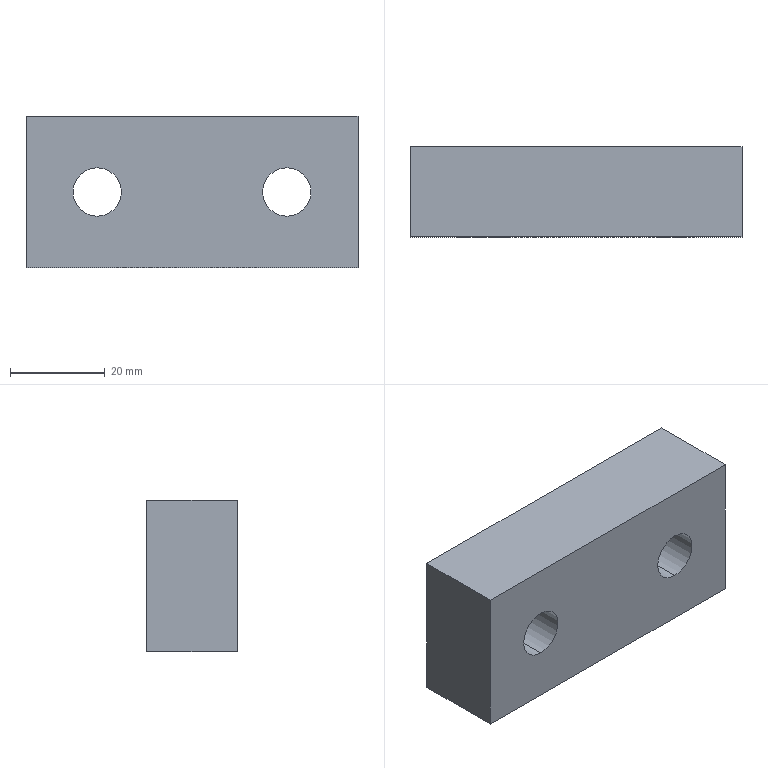Part | SolidWorks | features FlatPattern 1, HoleWzd 1, SMBaseFlange 1, SheetMetal 1 | 1 solid | 10 faces | box 70 x 19 x 32 mm | volume 39455 mm3 | plane 6 | cylinder 4 | commonest cylinder face diameters 10.2 x4
STEP:
#1=CARTESIAN_POINT('',(-20.,-19.,-5.1));
#2=VERTEX_POINT('',#1);
#3=CARTESIAN_POINT('',(-20.,-19.,5.1));
#4=VERTEX_POINT('',#3);
#5=CARTESIAN_POINT('',(-20.,-19.,0.));
#6=DIRECTION('',(0.,1.,0.));
#7=DIRECTION('',(0.,0.,1.));
#8=AXIS2_PLACEMENT_3D('',#5,#6,#7);
#9=CIRCLE('',#8,5.1);
#10=EDGE_CURVE('',#2,#4,#9,.T.);
#11=ORIENTED_EDGE('',*,*,#10,.F.);
#12=CARTESIAN_POINT('',(-20.,0.,-5.1));
#13=VERTEX_POINT('',#12);
#14=CARTESIAN_POINT('',(-20.,0.,-5.1));
#15=DIRECTION('',(0.,1.,0.));
#16=VECTOR('',#15,1000.);
#17=LINE('',#14,#16);
#18=EDGE_CURVE('',#2,#13,#17,.T.);
#19=ORIENTED_EDGE('',*,*,#18,.T.);
#20=CARTESIAN_POINT('',(-20.,0.,5.1));
#21=VERTEX_POINT('',#20);
#22=CARTESIAN_POINT('',(-20.,0.,0.));
#23=DIRECTION('',(0.,1.,0.));
#24=DIRECTION('',(0.,0.,1.));
#25=AXIS2_PLACEMENT_3D('',#22,#23,#24);
#26=CIRCLE('',#25,5.1);
#27=EDGE_CURVE('',#13,#21,#26,.T.);
#28=ORIENTED_EDGE('',*,*,#27,.T.);
#29=CARTESIAN_POINT('',(-20.,0.,5.1));
#30=DIRECTION('',(0.,1.,0.));
#31=VECTOR('',#30,1000.);
#32=LINE('',#29,#31);
#33=EDGE_CURVE('',#4,#21,#32,.T.);
#34=ORIENTED_EDGE('',*,*,#33,.F.);
#35=EDGE_LOOP('',(#11,#19,#28,#34));
#36=FACE_OUTER_BOUND('',#35,.T.);
#37=CARTESIAN_POINT('',(-20.,0.,0.));
#38=DIRECTION('',(0.,1.,0.));
#39=DIRECTION('',(0.,0.,1.));
#40=AXIS2_PLACEMENT_3D('',#37,#38,#39);
#41=CYLINDRICAL_SURFACE('',#40,5.1);
#42=ADVANCED_FACE('',(#36),#41,.F.);
#43=CARTESIAN_POINT('',(20.,-19.,-5.1));
#44=VERTEX_POINT('',#43);
#45=CARTESIAN_POINT('',(20.,-19.,5.1));
#46=VERTEX_POINT('',#45);
#47=CARTESIAN_POINT('',(20.,-19.,0.));
#48=DIRECTION('',(0.,1.,0.));
#49=DIRECTION('',(0.,0.,1.));
#50=AXIS2_PLACEMENT_3D('',#47,#48,#49);
#51=CIRCLE('',#50,5.1);
#52=EDGE_CURVE('',#44,#46,#51,.T.);
#53=ORIENTED_EDGE('',*,*,#52,.F.);
#54=CARTESIAN_POINT('',(20.,0.,-5.1));
#55=VERTEX_POINT('',#54);
#56=CARTESIAN_POINT('',(20.,0.,-5.1));
#57=DIRECTION('',(0.,1.,0.));
#58=VECTOR('',#57,1000.);
#59=LINE('',#56,#58);
#60=EDGE_CURVE('',#44,#55,#59,.T.);
#61=ORIENTED_EDGE('',*,*,#60,.T.);
#62=CARTESIAN_POINT('',(20.,0.,5.1));
#63=VERTEX_POINT('',#62);
#64=CARTESIAN_POINT('',(20.,0.,0.));
#65=DIRECTION('',(0.,1.,0.));
#66=DIRECTION('',(0.,0.,1.));
#67=AXIS2_PLACEMENT_3D('',#64,#65,#66);
#68=CIRCLE('',#67,5.1);
#69=EDGE_CURVE('',#55,#63,#68,.T.);
#70=ORIENTED_EDGE('',*,*,#69,.T.);
#71=CARTESIAN_POINT('',(20.,0.,5.1));
#72=DIRECTION('',(0.,1.,0.));
#73=VECTOR('',#72,1000.);
#74=LINE('',#71,#73);
#75=EDGE_CURVE('',#46,#63,#74,.T.);
#76=ORIENTED_EDGE('',*,*,#75,.F.);
#77=EDGE_LOOP('',(#53,#61,#70,#76));
#78=FACE_OUTER_BOUND('',#77,.T.);
#79=CARTESIAN_POINT('',(20.,0.,0.));
#80=DIRECTION('',(0.,1.,0.));
#81=DIRECTION('',(0.,0.,1.));
#82=AXIS2_PLACEMENT_3D('',#79,#80,#81);
#83=CYLINDRICAL_SURFACE('',#82,5.1);
#84=ADVANCED_FACE('',(#78),#83,.F.);
#85=CARTESIAN_POINT('',(35.,0.,16.));
#86=VERTEX_POINT('',#85);
#87=CARTESIAN_POINT('',(35.,0.,-16.));
#88=VERTEX_POINT('',#87);
#89=CARTESIAN_POINT('',(35.,0.,-16.));
#90=DIRECTION('',(0.,0.,-1.));
#91=VECTOR('',#90,1000.);
#92=LINE('',#89,#91);
#93=EDGE_CURVE('',#86,#88,#92,.T.);
#94=ORIENTED_EDGE('',*,*,#93,.F.);
#95=CARTESIAN_POINT('',(35.,-19.,16.));
#96=VERTEX_POINT('',#95);
#97=CARTESIAN_POINT('',(35.,-19.,16.));
#98=DIRECTION('',(0.,1.,0.));
#99=VECTOR('',#98,1000.);
#100=LINE('',#97,#99);
#101=EDGE_CURVE('',#96,#86,#100,.T.);
#102=ORIENTED_EDGE('',*,*,#101,.F.);
#103=CARTESIAN_POINT('',(35.,-19.,-16.));
#104=VERTEX_POINT('',#103);
#105=CARTESIAN_POINT('',(35.,-19.,-16.));
#106=DIRECTION('',(0.,0.,-1.));
#107=VECTOR('',#106,1000.);
#108=LINE('',#105,#107);
#109=EDGE_CURVE('',#96,#104,#108,.T.);
#110=ORIENTED_EDGE('',*,*,#109,.T.);
#111=CARTESIAN_POINT('',(35.,-19.,-16.));
#112=DIRECTION('',(0.,1.,0.));
#113=VECTOR('',#112,1000.);
#114=LINE('',#111,#113);
#115=EDGE_CURVE('',#104,#88,#114,.T.);
#116=ORIENTED_EDGE('',*,*,#115,.T.);
#117=EDGE_LOOP('',(#94,#102,#110,#116));
#118=FACE_OUTER_BOUND('',#117,.T.);
#119=CARTESIAN_POINT('',(35.,-19.,-16.));
#120=DIRECTION('',(1.,0.,0.));
#121=DIRECTION('',(0.,0.,-1.));
#122=AXIS2_PLACEMENT_3D('',#119,#120,#121);
#123=PLANE('',#122);
#124=ADVANCED_FACE('',(#118),#123,.T.);
#125=CARTESIAN_POINT('',(-35.,0.,16.));
#126=VERTEX_POINT('',#125);
#127=CARTESIAN_POINT('',(-35.,0.,16.));
#128=DIRECTION('',(1.,0.,0.));
#129=VECTOR('',#128,1000.);
#130=LINE('',#127,#129);
#131=EDGE_CURVE('',#126,#86,#130,.T.);
#132=ORIENTED_EDGE('',*,*,#131,.F.);
#133=CARTESIAN_POINT('',(-35.,-19.,16.));
#134=VERTEX_POINT('',#133);
#135=CARTESIAN_POINT('',(-35.,-19.,16.));
#136=DIRECTION('',(0.,1.,0.));
#137=VECTOR('',#136,1000.);
#138=LINE('',#135,#137);
#139=EDGE_CURVE('',#134,#126,#138,.T.);
#140=ORIENTED_EDGE('',*,*,#139,.F.);
#141=CARTESIAN_POINT('',(-35.,-19.,16.));
#142=DIRECTION('',(1.,0.,0.));
#143=VECTOR('',#142,1000.);
#144=LINE('',#141,#143);
#145=EDGE_CURVE('',#134,#96,#144,.T.);
#146=ORIENTED_EDGE('',*,*,#145,.T.);
#147=ORIENTED_EDGE('',*,*,#101,.T.);
#148=EDGE_LOOP('',(#132,#140,#146,#147));
#149=FACE_OUTER_BOUND('',#148,.T.);
#150=CARTESIAN_POINT('',(-35.,-19.,16.));
#151=DIRECTION('',(0.,0.,1.));
#152=DIRECTION('',(1.,0.,0.));
#153=AXIS2_PLACEMENT_3D('',#150,#151,#152);
#154=PLANE('',#153);
#155=ADVANCED_FACE('',(#149),#154,.T.);
#156=CARTESIAN_POINT('',(-35.,0.,-16.));
#157=VERTEX_POINT('',#156);
#158=CARTESIAN_POINT('',(-35.,0.,-16.));
#159=DIRECTION('',(0.,0.,1.));
#160=VECTOR('',#159,1000.);
#161=LINE('',#158,#160);
#162=EDGE_CURVE('',#157,#126,#161,.T.);
#163=ORIENTED_EDGE('',*,*,#162,.F.);
#164=CARTESIAN_POINT('',(-35.,-19.,-16.));
#165=VERTEX_POINT('',#164);
#166=CARTESIAN_POINT('',(-35.,-19.,-16.));
#167=DIRECTION('',(0.,1.,0.));
#168=VECTOR('',#167,1000.);
#169=LINE('',#166,#168);
#170=EDGE_CURVE('',#165,#157,#169,.T.);
#171=ORIENTED_EDGE('',*,*,#170,.F.);
#172=CARTESIAN_POINT('',(-35.,-19.,-16.));
#173=DIRECTION('',(0.,0.,1.));
#174=VECTOR('',#173,1000.);
#175=LINE('',#172,#174);
#176=EDGE_CURVE('',#165,#134,#175,.T.);
#177=ORIENTED_EDGE('',*,*,#176,.T.);
#178=ORIENTED_EDGE('',*,*,#139,.T.);
#179=EDGE_LOOP('',(#163,#171,#177,#178));
#180=FACE_OUTER_BOUND('',#179,.T.);
#181=CARTESIAN_POINT('',(-35.,-19.,-16.));
#182=DIRECTION('',(-1.,0.,0.));
#183=DIRECTION('',(0.,0.,1.));
#184=AXIS2_PLACEMENT_3D('',#181,#182,#183);
#185=PLANE('',#184);
#186=ADVANCED_FACE('',(#180),#185,.T.);
#187=CARTESIAN_POINT('',(-35.,0.,-16.));
#188=DIRECTION('',(-1.,0.,0.));
#189=VECTOR('',#188,1000.);
#190=LINE('',#187,#189);
#191=EDGE_CURVE('',#88,#157,#190,.T.);
#192=ORIENTED_EDGE('',*,*,#191,.F.);
#193=ORIENTED_EDGE('',*,*,#115,.F.);
#194=CARTESIAN_POINT('',(-35.,-19.,-16.));
#195=DIRECTION('',(-1.,0.,0.));
#196=VECTOR('',#195,1000.);
#197=LINE('',#194,#196);
#198=EDGE_CURVE('',#104,#165,#197,.T.);
#199=ORIENTED_EDGE('',*,*,#198,.T.);
#200=ORIENTED_EDGE('',*,*,#170,.T.);
#201=EDGE_LOOP('',(#192,#193,#199,#200));
#202=FACE_OUTER_BOUND('',#201,.T.);
#203=CARTESIAN_POINT('',(-35.,-19.,-16.));
#204=DIRECTION('',(0.,0.,-1.));
#205=DIRECTION('',(-1.,0.,0.));
#206=AXIS2_PLACEMENT_3D('',#203,#204,#205);
#207=PLANE('',#206);
#208=ADVANCED_FACE('',(#202),#207,.T.);
#209=CARTESIAN_POINT('',(-20.,-19.,0.));
#210=DIRECTION('',(0.,1.,0.));
#211=DIRECTION('',(0.,0.,1.));
#212=AXIS2_PLACEMENT_3D('',#209,#210,#211);
#213=CIRCLE('',#212,5.1);
#214=EDGE_CURVE('',#4,#2,#213,.T.);
#215=ORIENTED_EDGE('',*,*,#214,.T.);
#216=ORIENTED_EDGE('',*,*,#10,.T.);
#217=EDGE_LOOP('',(#215,#216));
#218=FACE_BOUND('',#217,.T.);
#219=CARTESIAN_POINT('',(20.,-19.,0.));
#220=DIRECTION('',(0.,1.,0.));
#221=DIRECTION('',(0.,0.,1.));
#222=AXIS2_PLACEMENT_3D('',#219,#220,#221);
#223=CIRCLE('',#222,5.1);
#224=EDGE_CURVE('',#46,#44,#223,.T.);
#225=ORIENTED_EDGE('',*,*,#224,.T.);
#226=ORIENTED_EDGE('',*,*,#52,.T.);
#227=EDGE_LOOP('',(#225,#226));
#228=FACE_BOUND('',#227,.T.);
#229=ORIENTED_EDGE('',*,*,#109,.F.);
#230=ORIENTED_EDGE('',*,*,#145,.F.);
#231=ORIENTED_EDGE('',*,*,#176,.F.);
#232=ORIENTED_EDGE('',*,*,#198,.F.);
#233=EDGE_LOOP('',(#229,#230,#231,#232));
#234=FACE_OUTER_BOUND('',#233,.T.);
#235=CARTESIAN_POINT('',(0.,-19.,0.));
#236=DIRECTION('',(0.,1.,0.));
#237=DIRECTION('',(0.,0.,1.));
#238=AXIS2_PLACEMENT_3D('',#235,#236,#237);
#239=PLANE('',#238);
#240=ADVANCED_FACE('',(#218,#228,#234),#239,.F.);
#241=CARTESIAN_POINT('',(-20.,0.,0.));
#242=DIRECTION('',(0.,1.,0.));
#243=DIRECTION('',(0.,0.,1.));
#244=AXIS2_PLACEMENT_3D('',#241,#242,#243);
#245=CIRCLE('',#244,5.1);
#246=EDGE_CURVE('',#21,#13,#245,.T.);
#247=ORIENTED_EDGE('',*,*,#246,.F.);
#248=ORIENTED_EDGE('',*,*,#27,.F.);
#249=EDGE_LOOP('',(#247,#248));
#250=FACE_BOUND('',#249,.T.);
#251=CARTESIAN_POINT('',(20.,0.,0.));
#252=DIRECTION('',(0.,1.,0.));
#253=DIRECTION('',(0.,0.,1.));
#254=AXIS2_PLACEMENT_3D('',#251,#252,#253);
#255=CIRCLE('',#254,5.1);
#256=EDGE_CURVE('',#63,#55,#255,.T.);
#257=ORIENTED_EDGE('',*,*,#256,.F.);
#258=ORIENTED_EDGE('',*,*,#69,.F.);
#259=EDGE_LOOP('',(#257,#258));
#260=FACE_BOUND('',#259,.T.);
#261=ORIENTED_EDGE('',*,*,#93,.T.);
#262=ORIENTED_EDGE('',*,*,#191,.T.);
#263=ORIENTED_EDGE('',*,*,#162,.T.);
#264=ORIENTED_EDGE('',*,*,#131,.T.);
#265=EDGE_LOOP('',(#261,#262,#263,#264));
#266=FACE_OUTER_BOUND('',#265,.T.);
#267=CARTESIAN_POINT('',(0.,0.,0.));
#268=DIRECTION('',(0.,1.,0.));
#269=DIRECTION('',(0.,0.,1.));
#270=AXIS2_PLACEMENT_3D('',#267,#268,#269);
#271=PLANE('',#270);
#272=ADVANCED_FACE('',(#250,#260,#266),#271,.T.);
#273=ORIENTED_EDGE('',*,*,#60,.F.);
#274=ORIENTED_EDGE('',*,*,#224,.F.);
#275=ORIENTED_EDGE('',*,*,#75,.T.);
#276=ORIENTED_EDGE('',*,*,#256,.T.);
#277=EDGE_LOOP('',(#273,#274,#275,#276));
#278=FACE_OUTER_BOUND('',#277,.T.);
#279=CARTESIAN_POINT('',(20.,0.,0.));
#280=DIRECTION('',(0.,1.,0.));
#281=DIRECTION('',(0.,0.,1.));
#282=AXIS2_PLACEMENT_3D('',#279,#280,#281);
#283=CYLINDRICAL_SURFACE('',#282,5.1);
#284=ADVANCED_FACE('',(#278),#283,.F.);
#285=ORIENTED_EDGE('',*,*,#18,.F.);
#286=ORIENTED_EDGE('',*,*,#214,.F.);
#287=ORIENTED_EDGE('',*,*,#33,.T.);
#288=ORIENTED_EDGE('',*,*,#246,.T.);
#289=EDGE_LOOP('',(#285,#286,#287,#288));
#290=FACE_OUTER_BOUND('',#289,.T.);
#291=CARTESIAN_POINT('',(-20.,0.,0.));
#292=DIRECTION('',(0.,1.,0.));
#293=DIRECTION('',(0.,0.,1.));
#294=AXIS2_PLACEMENT_3D('',#291,#292,#293);
#295=CYLINDRICAL_SURFACE('',#294,5.1);
#296=ADVANCED_FACE('',(#290),#295,.F.);
#297=CLOSED_SHELL('',(#42,#84,#124,#155,#186,#208,#240,#272,#284,#296));
#298=MANIFOLD_SOLID_BREP('',#297);
#299=CARTESIAN_POINT('',(0.,0.,0.));
#300=DIRECTION('',(0.,0.,1.));
#301=DIRECTION('',(1.,0.,0.));
#302=AXIS2_PLACEMENT_3D('',#299,#300,#301);
#303=(LENGTH_UNIT()NAMED_UNIT(*)SI_UNIT(.MILLI.,.METRE.));
#304=UNCERTAINTY_MEASURE_WITH_UNIT(LENGTH_MEASURE(0.00001),#303,'','');
#305=(NAMED_UNIT(*)PLANE_ANGLE_UNIT()SI_UNIT($,.RADIAN.));
#306=(NAMED_UNIT(*)SI_UNIT($,.STERADIAN.)SOLID_ANGLE_UNIT());
#307=(GEOMETRIC_REPRESENTATION_CONTEXT(3)GLOBAL_UNCERTAINTY_ASSIGNED_CONTEXT((#304))GLOBAL_UNIT_ASSIGNED_CONTEXT((#303,#305,#306))REPRESENTATION_CONTEXT('',''));
#308=ADVANCED_BREP_SHAPE_REPRESENTATION('',(#298,#302),#307);